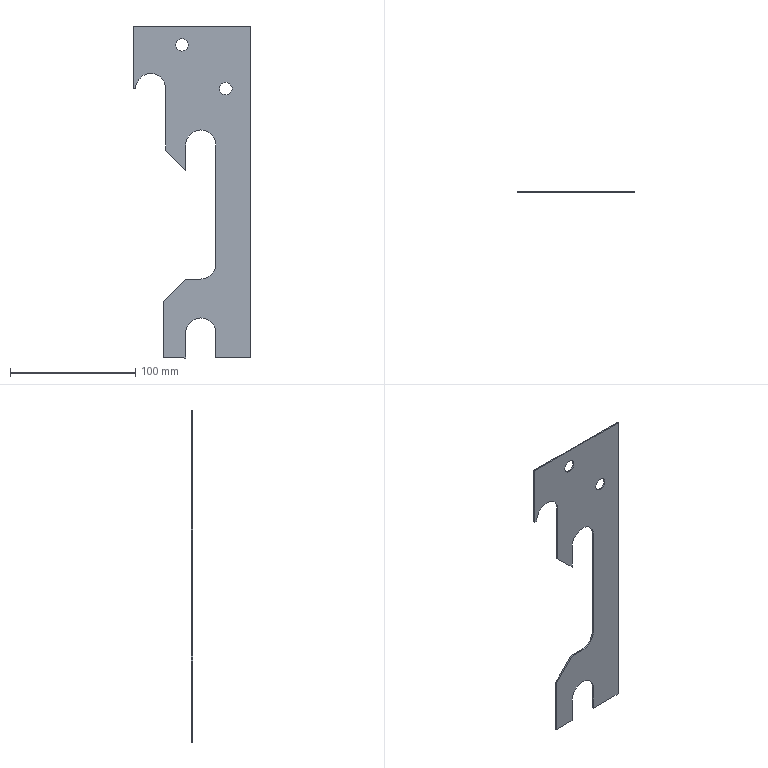Part | SolidWorks | features MirrorStock 1 | 1 solid | 28 faces | box 94 x 1 x 265 mm | volume 13911 mm3 | plane 17 | cylinder 11 | commonest cylinder face diameters 24 x7 10 x4
STEP:
#1=CARTESIAN_POINT('',(74.,1.,-5.));
#2=VERTEX_POINT('',#1);
#3=CARTESIAN_POINT('',(74.,1.,5.));
#4=VERTEX_POINT('',#3);
#5=CARTESIAN_POINT('',(74.,1.,0.));
#6=DIRECTION('',(0.,-1.,0.));
#7=DIRECTION('',(0.,0.,-1.));
#8=AXIS2_PLACEMENT_3D('',#5,#6,#7);
#9=CIRCLE('',#8,5.);
#10=EDGE_CURVE('',#2,#4,#9,.T.);
#11=ORIENTED_EDGE('',*,*,#10,.F.);
#12=CARTESIAN_POINT('',(74.,0.,-5.));
#13=VERTEX_POINT('',#12);
#14=CARTESIAN_POINT('',(74.,1.,-5.));
#15=DIRECTION('',(0.,-1.,0.));
#16=VECTOR('',#15,1000.);
#17=LINE('',#14,#16);
#18=EDGE_CURVE('',#2,#13,#17,.T.);
#19=ORIENTED_EDGE('',*,*,#18,.T.);
#20=CARTESIAN_POINT('',(74.,0.,5.));
#21=VERTEX_POINT('',#20);
#22=CARTESIAN_POINT('',(74.,0.,0.));
#23=DIRECTION('',(0.,-1.,0.));
#24=DIRECTION('',(0.,0.,-1.));
#25=AXIS2_PLACEMENT_3D('',#22,#23,#24);
#26=CIRCLE('',#25,5.);
#27=EDGE_CURVE('',#13,#21,#26,.T.);
#28=ORIENTED_EDGE('',*,*,#27,.T.);
#29=CARTESIAN_POINT('',(74.,1.,5.));
#30=DIRECTION('',(0.,-1.,0.));
#31=VECTOR('',#30,1000.);
#32=LINE('',#29,#31);
#33=EDGE_CURVE('',#4,#21,#32,.T.);
#34=ORIENTED_EDGE('',*,*,#33,.F.);
#35=EDGE_LOOP('',(#11,#19,#28,#34));
#36=FACE_OUTER_BOUND('',#35,.T.);
#37=CARTESIAN_POINT('',(74.,1.,0.));
#38=DIRECTION('',(0.,-1.,0.));
#39=DIRECTION('',(0.,0.,1.));
#40=AXIS2_PLACEMENT_3D('',#37,#38,#39);
#41=CYLINDRICAL_SURFACE('',#40,5.);
#42=ADVANCED_FACE('',(#36),#41,.F.);
#43=CARTESIAN_POINT('',(39.,1.,30.));
#44=VERTEX_POINT('',#43);
#45=CARTESIAN_POINT('',(39.,1.,40.));
#46=VERTEX_POINT('',#45);
#47=CARTESIAN_POINT('',(39.,1.,35.));
#48=DIRECTION('',(0.,-1.,0.));
#49=DIRECTION('',(0.,0.,-1.));
#50=AXIS2_PLACEMENT_3D('',#47,#48,#49);
#51=CIRCLE('',#50,5.);
#52=EDGE_CURVE('',#44,#46,#51,.T.);
#53=ORIENTED_EDGE('',*,*,#52,.F.);
#54=CARTESIAN_POINT('',(39.,0.,30.));
#55=VERTEX_POINT('',#54);
#56=CARTESIAN_POINT('',(39.,1.,30.));
#57=DIRECTION('',(0.,-1.,0.));
#58=VECTOR('',#57,1000.);
#59=LINE('',#56,#58);
#60=EDGE_CURVE('',#44,#55,#59,.T.);
#61=ORIENTED_EDGE('',*,*,#60,.T.);
#62=CARTESIAN_POINT('',(39.,0.,40.));
#63=VERTEX_POINT('',#62);
#64=CARTESIAN_POINT('',(39.,0.,35.));
#65=DIRECTION('',(0.,-1.,0.));
#66=DIRECTION('',(0.,0.,-1.));
#67=AXIS2_PLACEMENT_3D('',#64,#65,#66);
#68=CIRCLE('',#67,5.);
#69=EDGE_CURVE('',#55,#63,#68,.T.);
#70=ORIENTED_EDGE('',*,*,#69,.T.);
#71=CARTESIAN_POINT('',(39.,1.,40.));
#72=DIRECTION('',(0.,-1.,0.));
#73=VECTOR('',#72,1000.);
#74=LINE('',#71,#73);
#75=EDGE_CURVE('',#46,#63,#74,.T.);
#76=ORIENTED_EDGE('',*,*,#75,.F.);
#77=EDGE_LOOP('',(#53,#61,#70,#76));
#78=FACE_OUTER_BOUND('',#77,.T.);
#79=CARTESIAN_POINT('',(39.,1.,35.));
#80=DIRECTION('',(0.,-1.,0.));
#81=DIRECTION('',(0.,0.,1.));
#82=AXIS2_PLACEMENT_3D('',#79,#80,#81);
#83=CYLINDRICAL_SURFACE('',#82,5.);
#84=ADVANCED_FACE('',(#78),#83,.F.);
#85=CARTESIAN_POINT('',(42.,1.,-195.));
#86=VERTEX_POINT('',#85);
#87=CARTESIAN_POINT('',(54.,1.,-183.));
#88=VERTEX_POINT('',#87);
#89=CARTESIAN_POINT('',(54.,1.,-195.));
#90=DIRECTION('',(0.,1.,0.));
#91=DIRECTION('',(0.,0.,-1.));
#92=AXIS2_PLACEMENT_3D('',#89,#90,#91);
#93=CIRCLE('',#92,12.);
#94=EDGE_CURVE('',#86,#88,#93,.T.);
#95=ORIENTED_EDGE('',*,*,#94,.T.);
#96=CARTESIAN_POINT('',(54.,0.,-183.));
#97=VERTEX_POINT('',#96);
#98=CARTESIAN_POINT('',(54.,1.,-183.));
#99=DIRECTION('',(0.,-1.,0.));
#100=VECTOR('',#99,1000.);
#101=LINE('',#98,#100);
#102=EDGE_CURVE('',#88,#97,#101,.T.);
#103=ORIENTED_EDGE('',*,*,#102,.T.);
#104=CARTESIAN_POINT('',(42.,0.,-195.));
#105=VERTEX_POINT('',#104);
#106=CARTESIAN_POINT('',(54.,0.,-195.));
#107=DIRECTION('',(0.,1.,0.));
#108=DIRECTION('',(0.,0.,-1.));
#109=AXIS2_PLACEMENT_3D('',#106,#107,#108);
#110=CIRCLE('',#109,12.);
#111=EDGE_CURVE('',#105,#97,#110,.T.);
#112=ORIENTED_EDGE('',*,*,#111,.F.);
#113=CARTESIAN_POINT('',(42.,1.,-195.));
#114=DIRECTION('',(0.,-1.,0.));
#115=VECTOR('',#114,1000.);
#116=LINE('',#113,#115);
#117=EDGE_CURVE('',#86,#105,#116,.T.);
#118=ORIENTED_EDGE('',*,*,#117,.F.);
#119=EDGE_LOOP('',(#95,#103,#112,#118));
#120=FACE_OUTER_BOUND('',#119,.T.);
#121=CARTESIAN_POINT('',(54.,1.,-195.));
#122=DIRECTION('',(0.,-1.,0.));
#123=DIRECTION('',(0.,0.,1.));
#124=AXIS2_PLACEMENT_3D('',#121,#122,#123);
#125=CYLINDRICAL_SURFACE('',#124,12.);
#126=ADVANCED_FACE('',(#120),#125,.F.);
#127=CARTESIAN_POINT('',(42.,1.,-45.));
#128=VERTEX_POINT('',#127);
#129=CARTESIAN_POINT('',(54.,1.,-33.));
#130=VERTEX_POINT('',#129);
#131=CARTESIAN_POINT('',(54.,1.,-45.));
#132=DIRECTION('',(0.,1.,0.));
#133=DIRECTION('',(0.,0.,-1.));
#134=AXIS2_PLACEMENT_3D('',#131,#132,#133);
#135=CIRCLE('',#134,12.);
#136=EDGE_CURVE('',#128,#130,#135,.T.);
#137=ORIENTED_EDGE('',*,*,#136,.T.);
#138=CARTESIAN_POINT('',(54.,0.,-33.));
#139=VERTEX_POINT('',#138);
#140=CARTESIAN_POINT('',(54.,1.,-33.));
#141=DIRECTION('',(0.,-1.,0.));
#142=VECTOR('',#141,1000.);
#143=LINE('',#140,#142);
#144=EDGE_CURVE('',#130,#139,#143,.T.);
#145=ORIENTED_EDGE('',*,*,#144,.T.);
#146=CARTESIAN_POINT('',(42.,0.,-45.));
#147=VERTEX_POINT('',#146);
#148=CARTESIAN_POINT('',(54.,0.,-45.));
#149=DIRECTION('',(0.,1.,0.));
#150=DIRECTION('',(0.,0.,-1.));
#151=AXIS2_PLACEMENT_3D('',#148,#149,#150);
#152=CIRCLE('',#151,12.);
#153=EDGE_CURVE('',#147,#139,#152,.T.);
#154=ORIENTED_EDGE('',*,*,#153,.F.);
#155=CARTESIAN_POINT('',(42.,1.,-45.));
#156=DIRECTION('',(0.,-1.,0.));
#157=VECTOR('',#156,1000.);
#158=LINE('',#155,#157);
#159=EDGE_CURVE('',#128,#147,#158,.T.);
#160=ORIENTED_EDGE('',*,*,#159,.F.);
#161=EDGE_LOOP('',(#137,#145,#154,#160));
#162=FACE_OUTER_BOUND('',#161,.T.);
#163=CARTESIAN_POINT('',(54.,1.,-45.));
#164=DIRECTION('',(0.,-1.,0.));
#165=DIRECTION('',(0.,0.,1.));
#166=AXIS2_PLACEMENT_3D('',#163,#164,#165);
#167=CYLINDRICAL_SURFACE('',#166,12.);
#168=ADVANCED_FACE('',(#162),#167,.F.);
#169=CARTESIAN_POINT('',(2.,1.,0.));
#170=VERTEX_POINT('',#169);
#171=CARTESIAN_POINT('',(14.,1.,12.));
#172=VERTEX_POINT('',#171);
#173=CARTESIAN_POINT('',(14.,1.,0.));
#174=DIRECTION('',(0.,1.,0.));
#175=DIRECTION('',(0.,0.,-1.));
#176=AXIS2_PLACEMENT_3D('',#173,#174,#175);
#177=CIRCLE('',#176,12.);
#178=EDGE_CURVE('',#170,#172,#177,.T.);
#179=ORIENTED_EDGE('',*,*,#178,.T.);
#180=CARTESIAN_POINT('',(14.,0.,12.));
#181=VERTEX_POINT('',#180);
#182=CARTESIAN_POINT('',(14.,1.,12.));
#183=DIRECTION('',(0.,-1.,0.));
#184=VECTOR('',#183,1000.);
#185=LINE('',#182,#184);
#186=EDGE_CURVE('',#172,#181,#185,.T.);
#187=ORIENTED_EDGE('',*,*,#186,.T.);
#188=CARTESIAN_POINT('',(2.,0.,0.));
#189=VERTEX_POINT('',#188);
#190=CARTESIAN_POINT('',(14.,0.,0.));
#191=DIRECTION('',(0.,1.,0.));
#192=DIRECTION('',(0.,0.,-1.));
#193=AXIS2_PLACEMENT_3D('',#190,#191,#192);
#194=CIRCLE('',#193,12.);
#195=EDGE_CURVE('',#189,#181,#194,.T.);
#196=ORIENTED_EDGE('',*,*,#195,.F.);
#197=CARTESIAN_POINT('',(2.,1.,0.));
#198=DIRECTION('',(0.,-1.,0.));
#199=VECTOR('',#198,1000.);
#200=LINE('',#197,#199);
#201=EDGE_CURVE('',#170,#189,#200,.T.);
#202=ORIENTED_EDGE('',*,*,#201,.F.);
#203=EDGE_LOOP('',(#179,#187,#196,#202));
#204=FACE_OUTER_BOUND('',#203,.T.);
#205=CARTESIAN_POINT('',(14.,1.,0.));
#206=DIRECTION('',(0.,-1.,0.));
#207=DIRECTION('',(0.,0.,1.));
#208=AXIS2_PLACEMENT_3D('',#205,#206,#207);
#209=CYLINDRICAL_SURFACE('',#208,12.);
#210=ADVANCED_FACE('',(#204),#209,.F.);
#211=CARTESIAN_POINT('',(39.,1.,35.));
#212=DIRECTION('',(0.,-1.,0.));
#213=DIRECTION('',(0.,0.,-1.));
#214=AXIS2_PLACEMENT_3D('',#211,#212,#213);
#215=CIRCLE('',#214,5.);
#216=EDGE_CURVE('',#46,#44,#215,.T.);
#217=ORIENTED_EDGE('',*,*,#216,.T.);
#218=ORIENTED_EDGE('',*,*,#52,.T.);
#219=EDGE_LOOP('',(#217,#218));
#220=FACE_BOUND('',#219,.T.);
#221=CARTESIAN_POINT('',(0.,1.,0.));
#222=VERTEX_POINT('',#221);
#223=CARTESIAN_POINT('',(0.,1.,0.));
#224=DIRECTION('',(1.,0.,0.));
#225=VECTOR('',#224,1000.);
#226=LINE('',#223,#225);
#227=EDGE_CURVE('',#222,#170,#226,.T.);
#228=ORIENTED_EDGE('',*,*,#227,.F.);
#229=CARTESIAN_POINT('',(0.,1.,50.));
#230=VERTEX_POINT('',#229);
#231=CARTESIAN_POINT('',(0.,1.,0.));
#232=DIRECTION('',(0.,0.,-1.));
#233=VECTOR('',#232,1000.);
#234=LINE('',#231,#233);
#235=EDGE_CURVE('',#230,#222,#234,.T.);
#236=ORIENTED_EDGE('',*,*,#235,.F.);
#237=CARTESIAN_POINT('',(94.,1.,50.));
#238=VERTEX_POINT('',#237);
#239=CARTESIAN_POINT('',(0.,1.,50.));
#240=DIRECTION('',(-1.,0.,0.));
#241=VECTOR('',#240,1000.);
#242=LINE('',#239,#241);
#243=EDGE_CURVE('',#238,#230,#242,.T.);
#244=ORIENTED_EDGE('',*,*,#243,.F.);
#245=CARTESIAN_POINT('',(94.,1.,-215.));
#246=VERTEX_POINT('',#245);
#247=CARTESIAN_POINT('',(94.,1.,50.));
#248=DIRECTION('',(0.,0.,1.));
#249=VECTOR('',#248,1000.);
#250=LINE('',#247,#249);
#251=EDGE_CURVE('',#246,#238,#250,.T.);
#252=ORIENTED_EDGE('',*,*,#251,.F.);
#253=CARTESIAN_POINT('',(66.,1.,-215.));
#254=VERTEX_POINT('',#253);
#255=CARTESIAN_POINT('',(94.,1.,-215.));
#256=DIRECTION('',(1.,0.,0.));
#257=VECTOR('',#256,1000.);
#258=LINE('',#255,#257);
#259=EDGE_CURVE('',#254,#246,#258,.T.);
#260=ORIENTED_EDGE('',*,*,#259,.F.);
#261=CARTESIAN_POINT('',(66.,1.,-195.));
#262=VERTEX_POINT('',#261);
#263=CARTESIAN_POINT('',(66.,1.,-195.));
#264=DIRECTION('',(0.,0.,-1.));
#265=VECTOR('',#264,1000.);
#266=LINE('',#263,#265);
#267=EDGE_CURVE('',#262,#254,#266,.T.);
#268=ORIENTED_EDGE('',*,*,#267,.F.);
#269=CARTESIAN_POINT('',(54.,1.,-195.));
#270=DIRECTION('',(0.,1.,0.));
#271=DIRECTION('',(0.,0.,-1.));
#272=AXIS2_PLACEMENT_3D('',#269,#270,#271);
#273=CIRCLE('',#272,12.);
#274=EDGE_CURVE('',#88,#262,#273,.T.);
#275=ORIENTED_EDGE('',*,*,#274,.F.);
#276=ORIENTED_EDGE('',*,*,#94,.F.);
#277=CARTESIAN_POINT('',(42.,1.,-215.));
#278=VERTEX_POINT('',#277);
#279=CARTESIAN_POINT('',(42.,1.,-215.));
#280=DIRECTION('',(0.,0.,1.));
#281=VECTOR('',#280,1000.);
#282=LINE('',#279,#281);
#283=EDGE_CURVE('',#278,#86,#282,.T.);
#284=ORIENTED_EDGE('',*,*,#283,.F.);
#285=CARTESIAN_POINT('',(24.,1.,-215.));
#286=VERTEX_POINT('',#285);
#287=CARTESIAN_POINT('',(24.,1.,-215.));
#288=DIRECTION('',(1.,0.,0.));
#289=VECTOR('',#288,1000.);
#290=LINE('',#287,#289);
#291=EDGE_CURVE('',#286,#278,#290,.T.);
#292=ORIENTED_EDGE('',*,*,#291,.F.);
#293=CARTESIAN_POINT('',(24.,1.,-170.));
#294=VERTEX_POINT('',#293);
#295=CARTESIAN_POINT('',(24.,1.,-170.));
#296=DIRECTION('',(0.,0.,-1.));
#297=VECTOR('',#296,1000.);
#298=LINE('',#295,#297);
#299=EDGE_CURVE('',#294,#286,#298,.T.);
#300=ORIENTED_EDGE('',*,*,#299,.F.);
#301=CARTESIAN_POINT('',(42.,1.,-152.));
#302=VERTEX_POINT('',#301);
#303=CARTESIAN_POINT('',(42.,1.,-152.));
#304=DIRECTION('',(-0.7071,0.,-0.7071));
#305=VECTOR('',#304,1000.);
#306=LINE('',#303,#305);
#307=EDGE_CURVE('',#302,#294,#306,.T.);
#308=ORIENTED_EDGE('',*,*,#307,.F.);
#309=CARTESIAN_POINT('',(54.,1.,-152.));
#310=VERTEX_POINT('',#309);
#311=CARTESIAN_POINT('',(54.,1.,-152.));
#312=DIRECTION('',(-1.,0.,0.));
#313=VECTOR('',#312,1000.);
#314=LINE('',#311,#313);
#315=EDGE_CURVE('',#310,#302,#314,.T.);
#316=ORIENTED_EDGE('',*,*,#315,.F.);
#317=CARTESIAN_POINT('',(66.,1.,-140.));
#318=VERTEX_POINT('',#317);
#319=CARTESIAN_POINT('',(54.,1.,-140.));
#320=DIRECTION('',(0.,1.,0.));
#321=DIRECTION('',(0.,0.,1.));
#322=AXIS2_PLACEMENT_3D('',#319,#320,#321);
#323=CIRCLE('',#322,12.);
#324=EDGE_CURVE('',#318,#310,#323,.T.);
#325=ORIENTED_EDGE('',*,*,#324,.F.);
#326=CARTESIAN_POINT('',(66.,1.,-45.));
#327=VERTEX_POINT('',#326);
#328=CARTESIAN_POINT('',(66.,1.,-45.));
#329=DIRECTION('',(0.,0.,-1.));
#330=VECTOR('',#329,1000.);
#331=LINE('',#328,#330);
#332=EDGE_CURVE('',#327,#318,#331,.T.);
#333=ORIENTED_EDGE('',*,*,#332,.F.);
#334=CARTESIAN_POINT('',(54.,1.,-45.));
#335=DIRECTION('',(0.,1.,0.));
#336=DIRECTION('',(0.,0.,-1.));
#337=AXIS2_PLACEMENT_3D('',#334,#335,#336);
#338=CIRCLE('',#337,12.);
#339=EDGE_CURVE('',#130,#327,#338,.T.);
#340=ORIENTED_EDGE('',*,*,#339,.F.);
#341=ORIENTED_EDGE('',*,*,#136,.F.);
#342=CARTESIAN_POINT('',(42.,1.,-65.));
#343=VERTEX_POINT('',#342);
#344=CARTESIAN_POINT('',(42.,1.,-45.));
#345=DIRECTION('',(0.,0.,1.));
#346=VECTOR('',#345,1000.);
#347=LINE('',#344,#346);
#348=EDGE_CURVE('',#343,#128,#347,.T.);
#349=ORIENTED_EDGE('',*,*,#348,.F.);
#350=CARTESIAN_POINT('',(26.,1.,-49.));
#351=VERTEX_POINT('',#350);
#352=CARTESIAN_POINT('',(42.,1.,-65.));
#353=DIRECTION('',(0.7071,0.,-0.7071));
#354=VECTOR('',#353,1000.);
#355=LINE('',#352,#354);
#356=EDGE_CURVE('',#351,#343,#355,.T.);
#357=ORIENTED_EDGE('',*,*,#356,.F.);
#358=CARTESIAN_POINT('',(26.,1.,0.));
#359=VERTEX_POINT('',#358);
#360=CARTESIAN_POINT('',(26.,1.,-49.));
#361=DIRECTION('',(0.,0.,-1.));
#362=VECTOR('',#361,1000.);
#363=LINE('',#360,#362);
#364=EDGE_CURVE('',#359,#351,#363,.T.);
#365=ORIENTED_EDGE('',*,*,#364,.F.);
#366=CARTESIAN_POINT('',(14.,1.,0.));
#367=DIRECTION('',(0.,1.,0.));
#368=DIRECTION('',(0.,0.,-1.));
#369=AXIS2_PLACEMENT_3D('',#366,#367,#368);
#370=CIRCLE('',#369,12.);
#371=EDGE_CURVE('',#172,#359,#370,.T.);
#372=ORIENTED_EDGE('',*,*,#371,.F.);
#373=ORIENTED_EDGE('',*,*,#178,.F.);
#374=EDGE_LOOP('',(#228,#236,#244,#252,#260,#268,#275,#276,#284,#292,#300,#308,#316,#325,#333,#340,#341,#349,#357,#365,#372,#373));
#375=FACE_OUTER_BOUND('',#374,.T.);
#376=CARTESIAN_POINT('',(74.,1.,0.));
#377=DIRECTION('',(0.,-1.,0.));
#378=DIRECTION('',(0.,0.,-1.));
#379=AXIS2_PLACEMENT_3D('',#376,#377,#378);
#380=CIRCLE('',#379,5.);
#381=EDGE_CURVE('',#4,#2,#380,.T.);
#382=ORIENTED_EDGE('',*,*,#381,.T.);
#383=ORIENTED_EDGE('',*,*,#10,.T.);
#384=EDGE_LOOP('',(#382,#383));
#385=FACE_BOUND('',#384,.T.);
#386=CARTESIAN_POINT('',(14.,1.,0.));
#387=DIRECTION('',(0.,1.,0.));
#388=DIRECTION('',(0.,0.,-1.));
#389=AXIS2_PLACEMENT_3D('',#386,#387,#388);
#390=PLANE('',#389);
#391=ADVANCED_FACE('',(#220,#375,#385),#390,.T.);
#392=CARTESIAN_POINT('',(0.,0.,0.));
#393=VERTEX_POINT('',#392);
#394=CARTESIAN_POINT('',(0.,0.,0.));
#395=DIRECTION('',(1.,0.,0.));
#396=VECTOR('',#395,1000.);
#397=LINE('',#394,#396);
#398=EDGE_CURVE('',#393,#189,#397,.T.);
#399=ORIENTED_EDGE('',*,*,#398,.T.);
#400=ORIENTED_EDGE('',*,*,#195,.T.);
#401=CARTESIAN_POINT('',(26.,0.,0.));
#402=VERTEX_POINT('',#401);
#403=CARTESIAN_POINT('',(14.,0.,0.));
#404=DIRECTION('',(0.,1.,0.));
#405=DIRECTION('',(0.,0.,-1.));
#406=AXIS2_PLACEMENT_3D('',#403,#404,#405);
#407=CIRCLE('',#406,12.);
#408=EDGE_CURVE('',#181,#402,#407,.T.);
#409=ORIENTED_EDGE('',*,*,#408,.T.);
#410=CARTESIAN_POINT('',(26.,0.,-49.));
#411=VERTEX_POINT('',#410);
#412=CARTESIAN_POINT('',(26.,0.,-49.));
#413=DIRECTION('',(0.,0.,-1.));
#414=VECTOR('',#413,1000.);
#415=LINE('',#412,#414);
#416=EDGE_CURVE('',#402,#411,#415,.T.);
#417=ORIENTED_EDGE('',*,*,#416,.T.);
#418=CARTESIAN_POINT('',(42.,0.,-65.));
#419=VERTEX_POINT('',#418);
#420=CARTESIAN_POINT('',(42.,0.,-65.));
#421=DIRECTION('',(0.7071,0.,-0.7071));
#422=VECTOR('',#421,1000.);
#423=LINE('',#420,#422);
#424=EDGE_CURVE('',#411,#419,#423,.T.);
#425=ORIENTED_EDGE('',*,*,#424,.T.);
#426=CARTESIAN_POINT('',(42.,0.,-45.));
#427=DIRECTION('',(0.,0.,1.));
#428=VECTOR('',#427,1000.);
#429=LINE('',#426,#428);
#430=EDGE_CURVE('',#419,#147,#429,.T.);
#431=ORIENTED_EDGE('',*,*,#430,.T.);
#432=ORIENTED_EDGE('',*,*,#153,.T.);
#433=CARTESIAN_POINT('',(66.,0.,-45.));
#434=VERTEX_POINT('',#433);
#435=CARTESIAN_POINT('',(54.,0.,-45.));
#436=DIRECTION('',(0.,1.,0.));
#437=DIRECTION('',(0.,0.,-1.));
#438=AXIS2_PLACEMENT_3D('',#435,#436,#437);
#439=CIRCLE('',#438,12.);
#440=EDGE_CURVE('',#139,#434,#439,.T.);
#441=ORIENTED_EDGE('',*,*,#440,.T.);
#442=CARTESIAN_POINT('',(66.,0.,-140.));
#443=VERTEX_POINT('',#442);
#444=CARTESIAN_POINT('',(66.,0.,-45.));
#445=DIRECTION('',(0.,0.,-1.));
#446=VECTOR('',#445,1000.);
#447=LINE('',#444,#446);
#448=EDGE_CURVE('',#434,#443,#447,.T.);
#449=ORIENTED_EDGE('',*,*,#448,.T.);
#450=CARTESIAN_POINT('',(54.,0.,-152.));
#451=VERTEX_POINT('',#450);
#452=CARTESIAN_POINT('',(54.,0.,-140.));
#453=DIRECTION('',(0.,1.,0.));
#454=DIRECTION('',(0.,0.,1.));
#455=AXIS2_PLACEMENT_3D('',#452,#453,#454);
#456=CIRCLE('',#455,12.);
#457=EDGE_CURVE('',#443,#451,#456,.T.);
#458=ORIENTED_EDGE('',*,*,#457,.T.);
#459=CARTESIAN_POINT('',(42.,0.,-152.));
#460=VERTEX_POINT('',#459);
#461=CARTESIAN_POINT('',(54.,0.,-152.));
#462=DIRECTION('',(-1.,0.,0.));
#463=VECTOR('',#462,1000.);
#464=LINE('',#461,#463);
#465=EDGE_CURVE('',#451,#460,#464,.T.);
#466=ORIENTED_EDGE('',*,*,#465,.T.);
#467=CARTESIAN_POINT('',(24.,0.,-170.));
#468=VERTEX_POINT('',#467);
#469=CARTESIAN_POINT('',(42.,0.,-152.));
#470=DIRECTION('',(-0.7071,0.,-0.7071));
#471=VECTOR('',#470,1000.);
#472=LINE('',#469,#471);
#473=EDGE_CURVE('',#460,#468,#472,.T.);
#474=ORIENTED_EDGE('',*,*,#473,.T.);
#475=CARTESIAN_POINT('',(24.,0.,-215.));
#476=VERTEX_POINT('',#475);
#477=CARTESIAN_POINT('',(24.,0.,-170.));
#478=DIRECTION('',(0.,0.,-1.));
#479=VECTOR('',#478,1000.);
#480=LINE('',#477,#479);
#481=EDGE_CURVE('',#468,#476,#480,.T.);
#482=ORIENTED_EDGE('',*,*,#481,.T.);
#483=CARTESIAN_POINT('',(42.,0.,-215.));
#484=VERTEX_POINT('',#483);
#485=CARTESIAN_POINT('',(24.,0.,-215.));
#486=DIRECTION('',(1.,0.,0.));
#487=VECTOR('',#486,1000.);
#488=LINE('',#485,#487);
#489=EDGE_CURVE('',#476,#484,#488,.T.);
#490=ORIENTED_EDGE('',*,*,#489,.T.);
#491=CARTESIAN_POINT('',(42.,0.,-215.));
#492=DIRECTION('',(0.,0.,1.));
#493=VECTOR('',#492,1000.);
#494=LINE('',#491,#493);
#495=EDGE_CURVE('',#484,#105,#494,.T.);
#496=ORIENTED_EDGE('',*,*,#495,.T.);
#497=ORIENTED_EDGE('',*,*,#111,.T.);
#498=CARTESIAN_POINT('',(66.,0.,-195.));
#499=VERTEX_POINT('',#498);
#500=CARTESIAN_POINT('',(54.,0.,-195.));
#501=DIRECTION('',(0.,1.,0.));
#502=DIRECTION('',(0.,0.,-1.));
#503=AXIS2_PLACEMENT_3D('',#500,#501,#502);
#504=CIRCLE('',#503,12.);
#505=EDGE_CURVE('',#97,#499,#504,.T.);
#506=ORIENTED_EDGE('',*,*,#505,.T.);
#507=CARTESIAN_POINT('',(66.,0.,-215.));
#508=VERTEX_POINT('',#507);
#509=CARTESIAN_POINT('',(66.,0.,-195.));
#510=DIRECTION('',(0.,0.,-1.));
#511=VECTOR('',#510,1000.);
#512=LINE('',#509,#511);
#513=EDGE_CURVE('',#499,#508,#512,.T.);
#514=ORIENTED_EDGE('',*,*,#513,.T.);
#515=CARTESIAN_POINT('',(94.,0.,-215.));
#516=VERTEX_POINT('',#515);
#517=CARTESIAN_POINT('',(94.,0.,-215.));
#518=DIRECTION('',(1.,0.,0.));
#519=VECTOR('',#518,1000.);
#520=LINE('',#517,#519);
#521=EDGE_CURVE('',#508,#516,#520,.T.);
#522=ORIENTED_EDGE('',*,*,#521,.T.);
#523=CARTESIAN_POINT('',(94.,0.,50.));
#524=VERTEX_POINT('',#523);
#525=CARTESIAN_POINT('',(94.,0.,50.));
#526=DIRECTION('',(0.,0.,1.));
#527=VECTOR('',#526,1000.);
#528=LINE('',#525,#527);
#529=EDGE_CURVE('',#516,#524,#528,.T.);
#530=ORIENTED_EDGE('',*,*,#529,.T.);
#531=CARTESIAN_POINT('',(0.,0.,50.));
#532=VERTEX_POINT('',#531);
#533=CARTESIAN_POINT('',(0.,0.,50.));
#534=DIRECTION('',(-1.,0.,0.));
#535=VECTOR('',#534,1000.);
#536=LINE('',#533,#535);
#537=EDGE_CURVE('',#524,#532,#536,.T.);
#538=ORIENTED_EDGE('',*,*,#537,.T.);
#539=CARTESIAN_POINT('',(0.,0.,0.));
#540=DIRECTION('',(0.,0.,-1.));
#541=VECTOR('',#540,1000.);
#542=LINE('',#539,#541);
#543=EDGE_CURVE('',#532,#393,#542,.T.);
#544=ORIENTED_EDGE('',*,*,#543,.T.);
#545=EDGE_LOOP('',(#399,#400,#409,#417,#425,#431,#432,#441,#449,#458,#466,#474,#482,#490,#496,#497,#506,#514,#522,#530,#538,#544));
#546=FACE_OUTER_BOUND('',#545,.T.);
#547=CARTESIAN_POINT('',(39.,0.,35.));
#548=DIRECTION('',(0.,-1.,0.));
#549=DIRECTION('',(0.,0.,-1.));
#550=AXIS2_PLACEMENT_3D('',#547,#548,#549);
#551=CIRCLE('',#550,5.);
#552=EDGE_CURVE('',#63,#55,#551,.T.);
#553=ORIENTED_EDGE('',*,*,#552,.F.);
#554=ORIENTED_EDGE('',*,*,#69,.F.);
#555=EDGE_LOOP('',(#553,#554));
#556=FACE_BOUND('',#555,.T.);
#557=CARTESIAN_POINT('',(74.,0.,0.));
#558=DIRECTION('',(0.,-1.,0.));
#559=DIRECTION('',(0.,0.,-1.));
#560=AXIS2_PLACEMENT_3D('',#557,#558,#559);
#561=CIRCLE('',#560,5.);
#562=EDGE_CURVE('',#21,#13,#561,.T.);
#563=ORIENTED_EDGE('',*,*,#562,.F.);
#564=ORIENTED_EDGE('',*,*,#27,.F.);
#565=EDGE_LOOP('',(#563,#564));
#566=FACE_BOUND('',#565,.T.);
#567=CARTESIAN_POINT('',(14.,0.,0.));
#568=DIRECTION('',(0.,1.,0.));
#569=DIRECTION('',(0.,0.,-1.));
#570=AXIS2_PLACEMENT_3D('',#567,#568,#569);
#571=PLANE('',#570);
#572=ADVANCED_FACE('',(#546,#556,#566),#571,.F.);
#573=ORIENTED_EDGE('',*,*,#398,.F.);
#574=CARTESIAN_POINT('',(0.,1.,0.));
#575=DIRECTION('',(0.,-1.,0.));
#576=VECTOR('',#575,1000.);
#577=LINE('',#574,#576);
#578=EDGE_CURVE('',#222,#393,#577,.T.);
#579=ORIENTED_EDGE('',*,*,#578,.F.);
#580=ORIENTED_EDGE('',*,*,#227,.T.);
#581=ORIENTED_EDGE('',*,*,#201,.T.);
#582=EDGE_LOOP('',(#573,#579,#580,#581));
#583=FACE_OUTER_BOUND('',#582,.T.);
#584=CARTESIAN_POINT('',(0.,1.,0.));
#585=DIRECTION('',(0.,0.,1.));
#586=DIRECTION('',(-1.,0.,0.));
#587=AXIS2_PLACEMENT_3D('',#584,#585,#586);
#588=PLANE('',#587);
#589=ADVANCED_FACE('',(#583),#588,.F.);
#590=ORIENTED_EDGE('',*,*,#186,.F.);
#591=ORIENTED_EDGE('',*,*,#371,.T.);
#592=CARTESIAN_POINT('',(26.,1.,0.));
#593=DIRECTION('',(0.,-1.,0.));
#594=VECTOR('',#593,1000.);
#595=LINE('',#592,#594);
#596=EDGE_CURVE('',#359,#402,#595,.T.);
#597=ORIENTED_EDGE('',*,*,#596,.T.);
#598=ORIENTED_EDGE('',*,*,#408,.F.);
#599=EDGE_LOOP('',(#590,#591,#597,#598));
#600=FACE_OUTER_BOUND('',#599,.T.);
#601=CARTESIAN_POINT('',(14.,1.,0.));
#602=DIRECTION('',(0.,-1.,0.));
#603=DIRECTION('',(0.,0.,1.));
#604=AXIS2_PLACEMENT_3D('',#601,#602,#603);
#605=CYLINDRICAL_SURFACE('',#604,12.);
#606=ADVANCED_FACE('',(#600),#605,.F.);
#607=ORIENTED_EDGE('',*,*,#416,.F.);
#608=ORIENTED_EDGE('',*,*,#596,.F.);
#609=ORIENTED_EDGE('',*,*,#364,.T.);
#610=CARTESIAN_POINT('',(26.,1.,-49.));
#611=DIRECTION('',(0.,-1.,0.));
#612=VECTOR('',#611,1000.);
#613=LINE('',#610,#612);
#614=EDGE_CURVE('',#351,#411,#613,.T.);
#615=ORIENTED_EDGE('',*,*,#614,.T.);
#616=EDGE_LOOP('',(#607,#608,#609,#615));
#617=FACE_OUTER_BOUND('',#616,.T.);
#618=CARTESIAN_POINT('',(26.,1.,-49.));
#619=DIRECTION('',(1.,0.,0.));
#620=DIRECTION('',(0.,0.,1.));
#621=AXIS2_PLACEMENT_3D('',#618,#619,#620);
#622=PLANE('',#621);
#623=ADVANCED_FACE('',(#617),#622,.F.);
#624=ORIENTED_EDGE('',*,*,#424,.F.);
#625=ORIENTED_EDGE('',*,*,#614,.F.);
#626=ORIENTED_EDGE('',*,*,#356,.T.);
#627=CARTESIAN_POINT('',(42.,1.,-65.));
#628=DIRECTION('',(0.,-1.,0.));
#629=VECTOR('',#628,1000.);
#630=LINE('',#627,#629);
#631=EDGE_CURVE('',#343,#419,#630,.T.);
#632=ORIENTED_EDGE('',*,*,#631,.T.);
#633=EDGE_LOOP('',(#624,#625,#626,#632));
#634=FACE_OUTER_BOUND('',#633,.T.);
#635=CARTESIAN_POINT('',(42.,1.,-65.));
#636=DIRECTION('',(0.7071,0.,0.7071));
#637=DIRECTION('',(-0.7071,0.,0.7071));
#638=AXIS2_PLACEMENT_3D('',#635,#636,#637);
#639=PLANE('',#638);
#640=ADVANCED_FACE('',(#634),#639,.F.);
#641=ORIENTED_EDGE('',*,*,#430,.F.);
#642=ORIENTED_EDGE('',*,*,#631,.F.);
#643=ORIENTED_EDGE('',*,*,#348,.T.);
#644=ORIENTED_EDGE('',*,*,#159,.T.);
#645=EDGE_LOOP('',(#641,#642,#643,#644));
#646=FACE_OUTER_BOUND('',#645,.T.);
#647=CARTESIAN_POINT('',(42.,1.,-45.));
#648=DIRECTION('',(-1.,0.,0.));
#649=DIRECTION('',(0.,0.,-1.));
#650=AXIS2_PLACEMENT_3D('',#647,#648,#649);
#651=PLANE('',#650);
#652=ADVANCED_FACE('',(#646),#651,.F.);
#653=ORIENTED_EDGE('',*,*,#144,.F.);
#654=ORIENTED_EDGE('',*,*,#339,.T.);
#655=CARTESIAN_POINT('',(66.,1.,-45.));
#656=DIRECTION('',(0.,-1.,0.));
#657=VECTOR('',#656,1000.);
#658=LINE('',#655,#657);
#659=EDGE_CURVE('',#327,#434,#658,.T.);
#660=ORIENTED_EDGE('',*,*,#659,.T.);
#661=ORIENTED_EDGE('',*,*,#440,.F.);
#662=EDGE_LOOP('',(#653,#654,#660,#661));
#663=FACE_OUTER_BOUND('',#662,.T.);
#664=CARTESIAN_POINT('',(54.,1.,-45.));
#665=DIRECTION('',(0.,-1.,0.));
#666=DIRECTION('',(0.,0.,1.));
#667=AXIS2_PLACEMENT_3D('',#664,#665,#666);
#668=CYLINDRICAL_SURFACE('',#667,12.);
#669=ADVANCED_FACE('',(#663),#668,.F.);
#670=ORIENTED_EDGE('',*,*,#448,.F.);
#671=ORIENTED_EDGE('',*,*,#659,.F.);
#672=ORIENTED_EDGE('',*,*,#332,.T.);
#673=CARTESIAN_POINT('',(66.,1.,-140.));
#674=DIRECTION('',(0.,-1.,0.));
#675=VECTOR('',#674,1000.);
#676=LINE('',#673,#675);
#677=EDGE_CURVE('',#318,#443,#676,.T.);
#678=ORIENTED_EDGE('',*,*,#677,.T.);
#679=EDGE_LOOP('',(#670,#671,#672,#678));
#680=FACE_OUTER_BOUND('',#679,.T.);
#681=CARTESIAN_POINT('',(66.,1.,-45.));
#682=DIRECTION('',(1.,0.,0.));
#683=DIRECTION('',(0.,0.,1.));
#684=AXIS2_PLACEMENT_3D('',#681,#682,#683);
#685=PLANE('',#684);
#686=ADVANCED_FACE('',(#680),#685,.F.);
#687=ORIENTED_EDGE('',*,*,#457,.F.);
#688=ORIENTED_EDGE('',*,*,#677,.F.);
#689=ORIENTED_EDGE('',*,*,#324,.T.);
#690=CARTESIAN_POINT('',(54.,1.,-152.));
#691=DIRECTION('',(0.,-1.,0.));
#692=VECTOR('',#691,1000.);
#693=LINE('',#690,#692);
#694=EDGE_CURVE('',#310,#451,#693,.T.);
#695=ORIENTED_EDGE('',*,*,#694,.T.);
#696=EDGE_LOOP('',(#687,#688,#689,#695));
#697=FACE_OUTER_BOUND('',#696,.T.);
#698=CARTESIAN_POINT('',(54.,1.,-140.));
#699=DIRECTION('',(0.,-1.,0.));
#700=DIRECTION('',(0.,0.,1.));
#701=AXIS2_PLACEMENT_3D('',#698,#699,#700);
#702=CYLINDRICAL_SURFACE('',#701,12.);
#703=ADVANCED_FACE('',(#697),#702,.F.);
#704=ORIENTED_EDGE('',*,*,#465,.F.);
#705=ORIENTED_EDGE('',*,*,#694,.F.);
#706=ORIENTED_EDGE('',*,*,#315,.T.);
#707=CARTESIAN_POINT('',(42.,1.,-152.));
#708=DIRECTION('',(0.,-1.,0.));
#709=VECTOR('',#708,1000.);
#710=LINE('',#707,#709);
#711=EDGE_CURVE('',#302,#460,#710,.T.);
#712=ORIENTED_EDGE('',*,*,#711,.T.);
#713=EDGE_LOOP('',(#704,#705,#706,#712));
#714=FACE_OUTER_BOUND('',#713,.T.);
#715=CARTESIAN_POINT('',(54.,1.,-152.));
#716=DIRECTION('',(0.,0.,-1.));
#717=DIRECTION('',(1.,0.,0.));
#718=AXIS2_PLACEMENT_3D('',#715,#716,#717);
#719=PLANE('',#718);
#720=ADVANCED_FACE('',(#714),#719,.F.);
#721=ORIENTED_EDGE('',*,*,#473,.F.);
#722=ORIENTED_EDGE('',*,*,#711,.F.);
#723=ORIENTED_EDGE('',*,*,#307,.T.);
#724=CARTESIAN_POINT('',(24.,1.,-170.));
#725=DIRECTION('',(0.,-1.,0.));
#726=VECTOR('',#725,1000.);
#727=LINE('',#724,#726);
#728=EDGE_CURVE('',#294,#468,#727,.T.);
#729=ORIENTED_EDGE('',*,*,#728,.T.);
#730=EDGE_LOOP('',(#721,#722,#723,#729));
#731=FACE_OUTER_BOUND('',#730,.T.);
#732=CARTESIAN_POINT('',(42.,1.,-152.));
#733=DIRECTION('',(0.7071,0.,-0.7071));
#734=DIRECTION('',(0.7071,0.,0.7071));
#735=AXIS2_PLACEMENT_3D('',#732,#733,#734);
#736=PLANE('',#735);
#737=ADVANCED_FACE('',(#731),#736,.F.);
#738=ORIENTED_EDGE('',*,*,#481,.F.);
#739=ORIENTED_EDGE('',*,*,#728,.F.);
#740=ORIENTED_EDGE('',*,*,#299,.T.);
#741=CARTESIAN_POINT('',(24.,1.,-215.));
#742=DIRECTION('',(0.,-1.,0.));
#743=VECTOR('',#742,1000.);
#744=LINE('',#741,#743);
#745=EDGE_CURVE('',#286,#476,#744,.T.);
#746=ORIENTED_EDGE('',*,*,#745,.T.);
#747=EDGE_LOOP('',(#738,#739,#740,#746));
#748=FACE_OUTER_BOUND('',#747,.T.);
#749=CARTESIAN_POINT('',(24.,1.,-170.));
#750=DIRECTION('',(1.,0.,0.));
#751=DIRECTION('',(0.,0.,1.));
#752=AXIS2_PLACEMENT_3D('',#749,#750,#751);
#753=PLANE('',#752);
#754=ADVANCED_FACE('',(#748),#753,.F.);
#755=ORIENTED_EDGE('',*,*,#489,.F.);
#756=ORIENTED_EDGE('',*,*,#745,.F.);
#757=ORIENTED_EDGE('',*,*,#291,.T.);
#758=CARTESIAN_POINT('',(42.,1.,-215.));
#759=DIRECTION('',(0.,-1.,0.));
#760=VECTOR('',#759,1000.);
#761=LINE('',#758,#760);
#762=EDGE_CURVE('',#278,#484,#761,.T.);
#763=ORIENTED_EDGE('',*,*,#762,.T.);
#764=EDGE_LOOP('',(#755,#756,#757,#763));
#765=FACE_OUTER_BOUND('',#764,.T.);
#766=CARTESIAN_POINT('',(24.,1.,-215.));
#767=DIRECTION('',(0.,0.,1.));
#768=DIRECTION('',(-1.,0.,0.));
#769=AXIS2_PLACEMENT_3D('',#766,#767,#768);
#770=PLANE('',#769);
#771=ADVANCED_FACE('',(#765),#770,.F.);
#772=ORIENTED_EDGE('',*,*,#495,.F.);
#773=ORIENTED_EDGE('',*,*,#762,.F.);
#774=ORIENTED_EDGE('',*,*,#283,.T.);
#775=ORIENTED_EDGE('',*,*,#117,.T.);
#776=EDGE_LOOP('',(#772,#773,#774,#775));
#777=FACE_OUTER_BOUND('',#776,.T.);
#778=CARTESIAN_POINT('',(42.,1.,-215.));
#779=DIRECTION('',(-1.,0.,0.));
#780=DIRECTION('',(0.,0.,-1.));
#781=AXIS2_PLACEMENT_3D('',#778,#779,#780);
#782=PLANE('',#781);
#783=ADVANCED_FACE('',(#777),#782,.F.);
#784=ORIENTED_EDGE('',*,*,#102,.F.);
#785=ORIENTED_EDGE('',*,*,#274,.T.);
#786=CARTESIAN_POINT('',(66.,1.,-195.));
#787=DIRECTION('',(0.,-1.,0.));
#788=VECTOR('',#787,1000.);
#789=LINE('',#786,#788);
#790=EDGE_CURVE('',#262,#499,#789,.T.);
#791=ORIENTED_EDGE('',*,*,#790,.T.);
#792=ORIENTED_EDGE('',*,*,#505,.F.);
#793=EDGE_LOOP('',(#784,#785,#791,#792));
#794=FACE_OUTER_BOUND('',#793,.T.);
#795=CARTESIAN_POINT('',(54.,1.,-195.));
#796=DIRECTION('',(0.,-1.,0.));
#797=DIRECTION('',(0.,0.,1.));
#798=AXIS2_PLACEMENT_3D('',#795,#796,#797);
#799=CYLINDRICAL_SURFACE('',#798,12.);
#800=ADVANCED_FACE('',(#794),#799,.F.);
#801=ORIENTED_EDGE('',*,*,#513,.F.);
#802=ORIENTED_EDGE('',*,*,#790,.F.);
#803=ORIENTED_EDGE('',*,*,#267,.T.);
#804=CARTESIAN_POINT('',(66.,1.,-215.));
#805=DIRECTION('',(0.,-1.,0.));
#806=VECTOR('',#805,1000.);
#807=LINE('',#804,#806);
#808=EDGE_CURVE('',#254,#508,#807,.T.);
#809=ORIENTED_EDGE('',*,*,#808,.T.);
#810=EDGE_LOOP('',(#801,#802,#803,#809));
#811=FACE_OUTER_BOUND('',#810,.T.);
#812=CARTESIAN_POINT('',(66.,1.,-195.));
#813=DIRECTION('',(1.,0.,0.));
#814=DIRECTION('',(0.,0.,1.));
#815=AXIS2_PLACEMENT_3D('',#812,#813,#814);
#816=PLANE('',#815);
#817=ADVANCED_FACE('',(#811),#816,.F.);
#818=ORIENTED_EDGE('',*,*,#521,.F.);
#819=ORIENTED_EDGE('',*,*,#808,.F.);
#820=ORIENTED_EDGE('',*,*,#259,.T.);
#821=CARTESIAN_POINT('',(94.,1.,-215.));
#822=DIRECTION('',(0.,-1.,0.));
#823=VECTOR('',#822,1000.);
#824=LINE('',#821,#823);
#825=EDGE_CURVE('',#246,#516,#824,.T.);
#826=ORIENTED_EDGE('',*,*,#825,.T.);
#827=EDGE_LOOP('',(#818,#819,#820,#826));
#828=FACE_OUTER_BOUND('',#827,.T.);
#829=CARTESIAN_POINT('',(94.,1.,-215.));
#830=DIRECTION('',(0.,0.,1.));
#831=DIRECTION('',(-1.,0.,0.));
#832=AXIS2_PLACEMENT_3D('',#829,#830,#831);
#833=PLANE('',#832);
#834=ADVANCED_FACE('',(#828),#833,.F.);
#835=ORIENTED_EDGE('',*,*,#529,.F.);
#836=ORIENTED_EDGE('',*,*,#825,.F.);
#837=ORIENTED_EDGE('',*,*,#251,.T.);
#838=CARTESIAN_POINT('',(94.,1.,50.));
#839=DIRECTION('',(0.,-1.,0.));
#840=VECTOR('',#839,1000.);
#841=LINE('',#838,#840);
#842=EDGE_CURVE('',#238,#524,#841,.T.);
#843=ORIENTED_EDGE('',*,*,#842,.T.);
#844=EDGE_LOOP('',(#835,#836,#837,#843));
#845=FACE_OUTER_BOUND('',#844,.T.);
#846=CARTESIAN_POINT('',(94.,1.,50.));
#847=DIRECTION('',(-1.,0.,0.));
#848=DIRECTION('',(0.,0.,-1.));
#849=AXIS2_PLACEMENT_3D('',#846,#847,#848);
#850=PLANE('',#849);
#851=ADVANCED_FACE('',(#845),#850,.F.);
#852=ORIENTED_EDGE('',*,*,#537,.F.);
#853=ORIENTED_EDGE('',*,*,#842,.F.);
#854=ORIENTED_EDGE('',*,*,#243,.T.);
#855=CARTESIAN_POINT('',(0.,1.,50.));
#856=DIRECTION('',(0.,-1.,0.));
#857=VECTOR('',#856,1000.);
#858=LINE('',#855,#857);
#859=EDGE_CURVE('',#230,#532,#858,.T.);
#860=ORIENTED_EDGE('',*,*,#859,.T.);
#861=EDGE_LOOP('',(#852,#853,#854,#860));
#862=FACE_OUTER_BOUND('',#861,.T.);
#863=CARTESIAN_POINT('',(0.,1.,50.));
#864=DIRECTION('',(0.,0.,-1.));
#865=DIRECTION('',(1.,0.,0.));
#866=AXIS2_PLACEMENT_3D('',#863,#864,#865);
#867=PLANE('',#866);
#868=ADVANCED_FACE('',(#862),#867,.F.);
#869=ORIENTED_EDGE('',*,*,#543,.F.);
#870=ORIENTED_EDGE('',*,*,#859,.F.);
#871=ORIENTED_EDGE('',*,*,#235,.T.);
#872=ORIENTED_EDGE('',*,*,#578,.T.);
#873=EDGE_LOOP('',(#869,#870,#871,#872));
#874=FACE_OUTER_BOUND('',#873,.T.);
#875=CARTESIAN_POINT('',(0.,1.,0.));
#876=DIRECTION('',(1.,0.,0.));
#877=DIRECTION('',(0.,0.,1.));
#878=AXIS2_PLACEMENT_3D('',#875,#876,#877);
#879=PLANE('',#878);
#880=ADVANCED_FACE('',(#874),#879,.F.);
#881=ORIENTED_EDGE('',*,*,#60,.F.);
#882=ORIENTED_EDGE('',*,*,#216,.F.);
#883=ORIENTED_EDGE('',*,*,#75,.T.);
#884=ORIENTED_EDGE('',*,*,#552,.T.);
#885=EDGE_LOOP('',(#881,#882,#883,#884));
#886=FACE_OUTER_BOUND('',#885,.T.);
#887=CARTESIAN_POINT('',(39.,1.,35.));
#888=DIRECTION('',(0.,-1.,0.));
#889=DIRECTION('',(0.,0.,1.));
#890=AXIS2_PLACEMENT_3D('',#887,#888,#889);
#891=CYLINDRICAL_SURFACE('',#890,5.);
#892=ADVANCED_FACE('',(#886),#891,.F.);
#893=ORIENTED_EDGE('',*,*,#18,.F.);
#894=ORIENTED_EDGE('',*,*,#381,.F.);
#895=ORIENTED_EDGE('',*,*,#33,.T.);
#896=ORIENTED_EDGE('',*,*,#562,.T.);
#897=EDGE_LOOP('',(#893,#894,#895,#896));
#898=FACE_OUTER_BOUND('',#897,.T.);
#899=CARTESIAN_POINT('',(74.,1.,0.));
#900=DIRECTION('',(0.,-1.,0.));
#901=DIRECTION('',(0.,0.,1.));
#902=AXIS2_PLACEMENT_3D('',#899,#900,#901);
#903=CYLINDRICAL_SURFACE('',#902,5.);
#904=ADVANCED_FACE('',(#898),#903,.F.);
#905=CLOSED_SHELL('',(#42,#84,#126,#168,#210,#391,#572,#589,#606,#623,#640,#652,#669,#686,#703,#720,#737,#754,#771,#783,#800,#817,#834,#851,#868,#880,#892,#904));
#906=MANIFOLD_SOLID_BREP('',#905);
#907=CARTESIAN_POINT('',(0.,0.,0.));
#908=DIRECTION('',(0.,0.,1.));
#909=DIRECTION('',(1.,0.,0.));
#910=AXIS2_PLACEMENT_3D('',#907,#908,#909);
#911=(LENGTH_UNIT()NAMED_UNIT(*)SI_UNIT(.MILLI.,.METRE.));
#912=UNCERTAINTY_MEASURE_WITH_UNIT(LENGTH_MEASURE(0.00001),#911,'','');
#913=(NAMED_UNIT(*)PLANE_ANGLE_UNIT()SI_UNIT($,.RADIAN.));
#914=(NAMED_UNIT(*)SI_UNIT($,.STERADIAN.)SOLID_ANGLE_UNIT());
#915=(GEOMETRIC_REPRESENTATION_CONTEXT(3)GLOBAL_UNCERTAINTY_ASSIGNED_CONTEXT((#912))GLOBAL_UNIT_ASSIGNED_CONTEXT((#911,#913,#914))REPRESENTATION_CONTEXT('',''));
#916=ADVANCED_BREP_SHAPE_REPRESENTATION('',(#906,#910),#915);